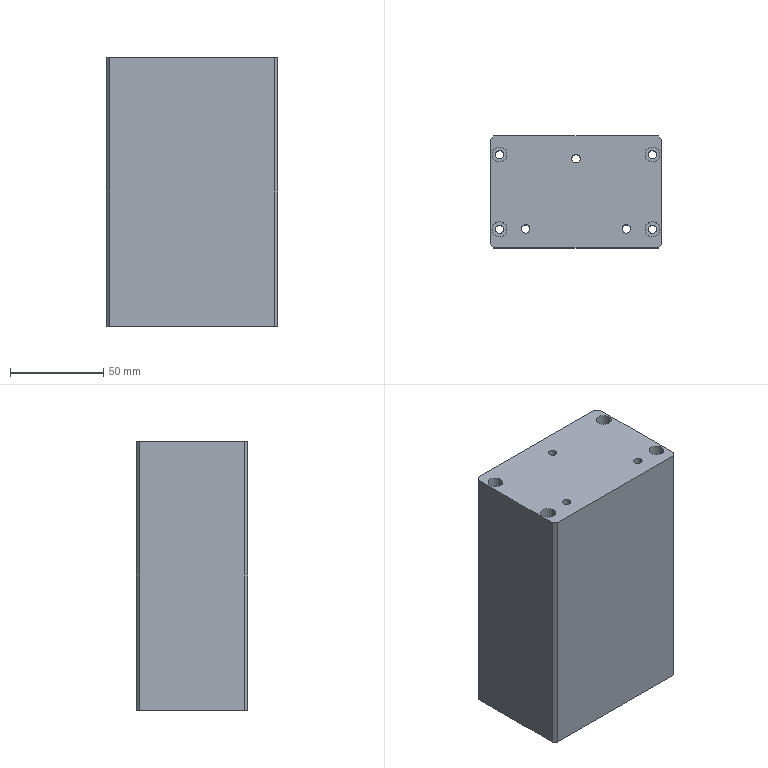Part | SolidWorks | features HoleWzd 2, Chamfer 1, Extrusion 1 | 1 solid | 45 faces | box 92 x 60 x 144 mm | volume 769072 mm3 | cylinder 28 | plane 17 | commonest cylinder face diameters 4.5 x14 8 x14
STEP:
#1=CARTESIAN_POINT('',(4.,17.7,37.));
#2=VERTEX_POINT('',#1);
#3=CARTESIAN_POINT('',(-4.,17.7,37.));
#4=VERTEX_POINT('',#3);
#5=CARTESIAN_POINT('',(0.,17.7,37.));
#6=DIRECTION('',(0.,0.,-1.));
#7=DIRECTION('',(-1.,0.,0.));
#8=AXIS2_PLACEMENT_3D('',#5,#6,#7);
#9=CIRCLE('',#8,4.);
#10=EDGE_CURVE('',#2,#4,#9,.T.);
#11=ORIENTED_EDGE('',*,*,#10,.F.);
#12=CARTESIAN_POINT('',(4.,17.7,0.));
#13=VERTEX_POINT('',#12);
#14=CARTESIAN_POINT('',(4.,17.7,0.));
#15=DIRECTION('',(0.,0.,-1.));
#16=VECTOR('',#15,1000.);
#17=LINE('',#14,#16);
#18=EDGE_CURVE('',#2,#13,#17,.T.);
#19=ORIENTED_EDGE('',*,*,#18,.T.);
#20=CARTESIAN_POINT('',(-4.,17.7,0.));
#21=VERTEX_POINT('',#20);
#22=CARTESIAN_POINT('',(0.,17.7,0.));
#23=DIRECTION('',(0.,0.,-1.));
#24=DIRECTION('',(-1.,0.,0.));
#25=AXIS2_PLACEMENT_3D('',#22,#23,#24);
#26=CIRCLE('',#25,4.);
#27=EDGE_CURVE('',#13,#21,#26,.T.);
#28=ORIENTED_EDGE('',*,*,#27,.T.);
#29=CARTESIAN_POINT('',(-4.,17.7,0.));
#30=DIRECTION('',(0.,0.,-1.));
#31=VECTOR('',#30,1000.);
#32=LINE('',#29,#31);
#33=EDGE_CURVE('',#4,#21,#32,.T.);
#34=ORIENTED_EDGE('',*,*,#33,.F.);
#35=EDGE_LOOP('',(#11,#19,#28,#34));
#36=FACE_OUTER_BOUND('',#35,.T.);
#37=CARTESIAN_POINT('',(0.,17.7,0.));
#38=DIRECTION('',(0.,0.,-1.));
#39=DIRECTION('',(-1.,0.,0.));
#40=AXIS2_PLACEMENT_3D('',#37,#38,#39);
#41=CYLINDRICAL_SURFACE('',#40,4.);
#42=ADVANCED_FACE('',(#36),#41,.F.);
#43=CARTESIAN_POINT('',(2.25,17.7,144.));
#44=VERTEX_POINT('',#43);
#45=CARTESIAN_POINT('',(-2.25,17.7,144.));
#46=VERTEX_POINT('',#45);
#47=CARTESIAN_POINT('',(0.,17.7,144.));
#48=DIRECTION('',(0.,0.,-1.));
#49=DIRECTION('',(-1.,0.,0.));
#50=AXIS2_PLACEMENT_3D('',#47,#48,#49);
#51=CIRCLE('',#50,2.25);
#52=EDGE_CURVE('',#44,#46,#51,.T.);
#53=ORIENTED_EDGE('',*,*,#52,.F.);
#54=CARTESIAN_POINT('',(2.25,17.7,37.));
#55=VERTEX_POINT('',#54);
#56=CARTESIAN_POINT('',(2.25,17.7,0.));
#57=DIRECTION('',(0.,0.,-1.));
#58=VECTOR('',#57,1000.);
#59=LINE('',#56,#58);
#60=EDGE_CURVE('',#44,#55,#59,.T.);
#61=ORIENTED_EDGE('',*,*,#60,.T.);
#62=CARTESIAN_POINT('',(-2.25,17.7,37.));
#63=VERTEX_POINT('',#62);
#64=CARTESIAN_POINT('',(0.,17.7,37.));
#65=DIRECTION('',(0.,0.,-1.));
#66=DIRECTION('',(-1.,0.,0.));
#67=AXIS2_PLACEMENT_3D('',#64,#65,#66);
#68=CIRCLE('',#67,2.25);
#69=EDGE_CURVE('',#55,#63,#68,.T.);
#70=ORIENTED_EDGE('',*,*,#69,.T.);
#71=CARTESIAN_POINT('',(-2.25,17.7,0.));
#72=DIRECTION('',(0.,0.,-1.));
#73=VECTOR('',#72,1000.);
#74=LINE('',#71,#73);
#75=EDGE_CURVE('',#46,#63,#74,.T.);
#76=ORIENTED_EDGE('',*,*,#75,.F.);
#77=EDGE_LOOP('',(#53,#61,#70,#76));
#78=FACE_OUTER_BOUND('',#77,.T.);
#79=CARTESIAN_POINT('',(0.,17.7,0.));
#80=DIRECTION('',(0.,0.,-1.));
#81=DIRECTION('',(-1.,0.,0.));
#82=AXIS2_PLACEMENT_3D('',#79,#80,#81);
#83=CYLINDRICAL_SURFACE('',#82,2.25);
#84=ADVANCED_FACE('',(#78),#83,.F.);
#85=CARTESIAN_POINT('',(31.,-19.9,37.));
#86=VERTEX_POINT('',#85);
#87=CARTESIAN_POINT('',(23.,-19.9,37.));
#88=VERTEX_POINT('',#87);
#89=CARTESIAN_POINT('',(27.,-19.9,37.));
#90=DIRECTION('',(0.,0.,-1.));
#91=DIRECTION('',(-1.,0.,0.));
#92=AXIS2_PLACEMENT_3D('',#89,#90,#91);
#93=CIRCLE('',#92,4.);
#94=EDGE_CURVE('',#86,#88,#93,.T.);
#95=ORIENTED_EDGE('',*,*,#94,.F.);
#96=CARTESIAN_POINT('',(31.,-19.9,0.));
#97=VERTEX_POINT('',#96);
#98=CARTESIAN_POINT('',(31.,-19.9,0.));
#99=DIRECTION('',(0.,0.,-1.));
#100=VECTOR('',#99,1000.);
#101=LINE('',#98,#100);
#102=EDGE_CURVE('',#86,#97,#101,.T.);
#103=ORIENTED_EDGE('',*,*,#102,.T.);
#104=CARTESIAN_POINT('',(23.,-19.9,0.));
#105=VERTEX_POINT('',#104);
#106=CARTESIAN_POINT('',(27.,-19.9,0.));
#107=DIRECTION('',(0.,0.,-1.));
#108=DIRECTION('',(-1.,0.,0.));
#109=AXIS2_PLACEMENT_3D('',#106,#107,#108);
#110=CIRCLE('',#109,4.);
#111=EDGE_CURVE('',#97,#105,#110,.T.);
#112=ORIENTED_EDGE('',*,*,#111,.T.);
#113=CARTESIAN_POINT('',(23.,-19.9,0.));
#114=DIRECTION('',(0.,0.,-1.));
#115=VECTOR('',#114,1000.);
#116=LINE('',#113,#115);
#117=EDGE_CURVE('',#88,#105,#116,.T.);
#118=ORIENTED_EDGE('',*,*,#117,.F.);
#119=EDGE_LOOP('',(#95,#103,#112,#118));
#120=FACE_OUTER_BOUND('',#119,.T.);
#121=CARTESIAN_POINT('',(27.,-19.9,0.));
#122=DIRECTION('',(0.,0.,-1.));
#123=DIRECTION('',(-1.,0.,0.));
#124=AXIS2_PLACEMENT_3D('',#121,#122,#123);
#125=CYLINDRICAL_SURFACE('',#124,4.);
#126=ADVANCED_FACE('',(#120),#125,.F.);
#127=CARTESIAN_POINT('',(29.25,-19.9,144.));
#128=VERTEX_POINT('',#127);
#129=CARTESIAN_POINT('',(24.75,-19.9,144.));
#130=VERTEX_POINT('',#129);
#131=CARTESIAN_POINT('',(27.,-19.9,144.));
#132=DIRECTION('',(0.,0.,-1.));
#133=DIRECTION('',(-1.,0.,0.));
#134=AXIS2_PLACEMENT_3D('',#131,#132,#133);
#135=CIRCLE('',#134,2.25);
#136=EDGE_CURVE('',#128,#130,#135,.T.);
#137=ORIENTED_EDGE('',*,*,#136,.F.);
#138=CARTESIAN_POINT('',(29.25,-19.9,37.));
#139=VERTEX_POINT('',#138);
#140=CARTESIAN_POINT('',(29.25,-19.9,0.));
#141=DIRECTION('',(0.,0.,-1.));
#142=VECTOR('',#141,1000.);
#143=LINE('',#140,#142);
#144=EDGE_CURVE('',#128,#139,#143,.T.);
#145=ORIENTED_EDGE('',*,*,#144,.T.);
#146=CARTESIAN_POINT('',(24.75,-19.9,37.));
#147=VERTEX_POINT('',#146);
#148=CARTESIAN_POINT('',(27.,-19.9,37.));
#149=DIRECTION('',(0.,0.,-1.));
#150=DIRECTION('',(-1.,0.,0.));
#151=AXIS2_PLACEMENT_3D('',#148,#149,#150);
#152=CIRCLE('',#151,2.25);
#153=EDGE_CURVE('',#139,#147,#152,.T.);
#154=ORIENTED_EDGE('',*,*,#153,.T.);
#155=CARTESIAN_POINT('',(24.75,-19.9,0.));
#156=DIRECTION('',(0.,0.,-1.));
#157=VECTOR('',#156,1000.);
#158=LINE('',#155,#157);
#159=EDGE_CURVE('',#130,#147,#158,.T.);
#160=ORIENTED_EDGE('',*,*,#159,.F.);
#161=EDGE_LOOP('',(#137,#145,#154,#160));
#162=FACE_OUTER_BOUND('',#161,.T.);
#163=CARTESIAN_POINT('',(27.,-19.9,0.));
#164=DIRECTION('',(0.,0.,-1.));
#165=DIRECTION('',(-1.,0.,0.));
#166=AXIS2_PLACEMENT_3D('',#163,#164,#165);
#167=CYLINDRICAL_SURFACE('',#166,2.25);
#168=ADVANCED_FACE('',(#162),#167,.F.);
#169=CARTESIAN_POINT('',(-23.,-19.9,37.));
#170=VERTEX_POINT('',#169);
#171=CARTESIAN_POINT('',(-31.,-19.9,37.));
#172=VERTEX_POINT('',#171);
#173=CARTESIAN_POINT('',(-27.,-19.9,37.));
#174=DIRECTION('',(0.,0.,-1.));
#175=DIRECTION('',(-1.,0.,0.));
#176=AXIS2_PLACEMENT_3D('',#173,#174,#175);
#177=CIRCLE('',#176,4.);
#178=EDGE_CURVE('',#170,#172,#177,.T.);
#179=ORIENTED_EDGE('',*,*,#178,.F.);
#180=CARTESIAN_POINT('',(-23.,-19.9,0.));
#181=VERTEX_POINT('',#180);
#182=CARTESIAN_POINT('',(-23.,-19.9,0.));
#183=DIRECTION('',(0.,0.,-1.));
#184=VECTOR('',#183,1000.);
#185=LINE('',#182,#184);
#186=EDGE_CURVE('',#170,#181,#185,.T.);
#187=ORIENTED_EDGE('',*,*,#186,.T.);
#188=CARTESIAN_POINT('',(-31.,-19.9,0.));
#189=VERTEX_POINT('',#188);
#190=CARTESIAN_POINT('',(-27.,-19.9,0.));
#191=DIRECTION('',(0.,0.,-1.));
#192=DIRECTION('',(-1.,0.,0.));
#193=AXIS2_PLACEMENT_3D('',#190,#191,#192);
#194=CIRCLE('',#193,4.);
#195=EDGE_CURVE('',#181,#189,#194,.T.);
#196=ORIENTED_EDGE('',*,*,#195,.T.);
#197=CARTESIAN_POINT('',(-31.,-19.9,0.));
#198=DIRECTION('',(0.,0.,-1.));
#199=VECTOR('',#198,1000.);
#200=LINE('',#197,#199);
#201=EDGE_CURVE('',#172,#189,#200,.T.);
#202=ORIENTED_EDGE('',*,*,#201,.F.);
#203=EDGE_LOOP('',(#179,#187,#196,#202));
#204=FACE_OUTER_BOUND('',#203,.T.);
#205=CARTESIAN_POINT('',(-27.,-19.9,0.));
#206=DIRECTION('',(0.,0.,-1.));
#207=DIRECTION('',(-1.,0.,0.));
#208=AXIS2_PLACEMENT_3D('',#205,#206,#207);
#209=CYLINDRICAL_SURFACE('',#208,4.);
#210=ADVANCED_FACE('',(#204),#209,.F.);
#211=CARTESIAN_POINT('',(-24.75,-19.9,144.));
#212=VERTEX_POINT('',#211);
#213=CARTESIAN_POINT('',(-29.25,-19.9,144.));
#214=VERTEX_POINT('',#213);
#215=CARTESIAN_POINT('',(-27.,-19.9,144.));
#216=DIRECTION('',(0.,0.,-1.));
#217=DIRECTION('',(-1.,0.,0.));
#218=AXIS2_PLACEMENT_3D('',#215,#216,#217);
#219=CIRCLE('',#218,2.25);
#220=EDGE_CURVE('',#212,#214,#219,.T.);
#221=ORIENTED_EDGE('',*,*,#220,.F.);
#222=CARTESIAN_POINT('',(-24.75,-19.9,37.));
#223=VERTEX_POINT('',#222);
#224=CARTESIAN_POINT('',(-24.75,-19.9,0.));
#225=DIRECTION('',(0.,0.,-1.));
#226=VECTOR('',#225,1000.);
#227=LINE('',#224,#226);
#228=EDGE_CURVE('',#212,#223,#227,.T.);
#229=ORIENTED_EDGE('',*,*,#228,.T.);
#230=CARTESIAN_POINT('',(-29.25,-19.9,37.));
#231=VERTEX_POINT('',#230);
#232=CARTESIAN_POINT('',(-27.,-19.9,37.));
#233=DIRECTION('',(0.,0.,-1.));
#234=DIRECTION('',(-1.,0.,0.));
#235=AXIS2_PLACEMENT_3D('',#232,#233,#234);
#236=CIRCLE('',#235,2.25);
#237=EDGE_CURVE('',#223,#231,#236,.T.);
#238=ORIENTED_EDGE('',*,*,#237,.T.);
#239=CARTESIAN_POINT('',(-29.25,-19.9,0.));
#240=DIRECTION('',(0.,0.,-1.));
#241=VECTOR('',#240,1000.);
#242=LINE('',#239,#241);
#243=EDGE_CURVE('',#214,#231,#242,.T.);
#244=ORIENTED_EDGE('',*,*,#243,.F.);
#245=EDGE_LOOP('',(#221,#229,#238,#244));
#246=FACE_OUTER_BOUND('',#245,.T.);
#247=CARTESIAN_POINT('',(-27.,-19.9,0.));
#248=DIRECTION('',(0.,0.,-1.));
#249=DIRECTION('',(-1.,0.,0.));
#250=AXIS2_PLACEMENT_3D('',#247,#248,#249);
#251=CYLINDRICAL_SURFACE('',#250,2.25);
#252=ADVANCED_FACE('',(#246),#251,.F.);
#253=CARTESIAN_POINT('',(-45.,20.,109.));
#254=VERTEX_POINT('',#253);
#255=CARTESIAN_POINT('',(-37.,20.,109.));
#256=VERTEX_POINT('',#255);
#257=CARTESIAN_POINT('',(-41.,20.,109.));
#258=DIRECTION('',(0.,0.,1.));
#259=DIRECTION('',(1.,0.,0.));
#260=AXIS2_PLACEMENT_3D('',#257,#258,#259);
#261=CIRCLE('',#260,4.);
#262=EDGE_CURVE('',#254,#256,#261,.T.);
#263=ORIENTED_EDGE('',*,*,#262,.F.);
#264=CARTESIAN_POINT('',(-45.,20.,144.));
#265=VERTEX_POINT('',#264);
#266=CARTESIAN_POINT('',(-45.,20.,144.));
#267=DIRECTION('',(0.,0.,1.));
#268=VECTOR('',#267,1000.);
#269=LINE('',#266,#268);
#270=EDGE_CURVE('',#254,#265,#269,.T.);
#271=ORIENTED_EDGE('',*,*,#270,.T.);
#272=CARTESIAN_POINT('',(-37.,20.,144.));
#273=VERTEX_POINT('',#272);
#274=CARTESIAN_POINT('',(-41.,20.,144.));
#275=DIRECTION('',(0.,0.,1.));
#276=DIRECTION('',(1.,0.,0.));
#277=AXIS2_PLACEMENT_3D('',#274,#275,#276);
#278=CIRCLE('',#277,4.);
#279=EDGE_CURVE('',#265,#273,#278,.T.);
#280=ORIENTED_EDGE('',*,*,#279,.T.);
#281=CARTESIAN_POINT('',(-37.,20.,144.));
#282=DIRECTION('',(0.,0.,1.));
#283=VECTOR('',#282,1000.);
#284=LINE('',#281,#283);
#285=EDGE_CURVE('',#256,#273,#284,.T.);
#286=ORIENTED_EDGE('',*,*,#285,.F.);
#287=EDGE_LOOP('',(#263,#271,#280,#286));
#288=FACE_OUTER_BOUND('',#287,.T.);
#289=CARTESIAN_POINT('',(-41.,20.,144.));
#290=DIRECTION('',(0.,0.,1.));
#291=DIRECTION('',(1.,0.,0.));
#292=AXIS2_PLACEMENT_3D('',#289,#290,#291);
#293=CYLINDRICAL_SURFACE('',#292,4.);
#294=ADVANCED_FACE('',(#288),#293,.F.);
#295=CARTESIAN_POINT('',(-43.25,20.,0.));
#296=VERTEX_POINT('',#295);
#297=CARTESIAN_POINT('',(-38.75,20.,0.));
#298=VERTEX_POINT('',#297);
#299=CARTESIAN_POINT('',(-41.,20.,0.));
#300=DIRECTION('',(0.,0.,1.));
#301=DIRECTION('',(1.,0.,0.));
#302=AXIS2_PLACEMENT_3D('',#299,#300,#301);
#303=CIRCLE('',#302,2.25);
#304=EDGE_CURVE('',#296,#298,#303,.T.);
#305=ORIENTED_EDGE('',*,*,#304,.F.);
#306=CARTESIAN_POINT('',(-43.25,20.,109.));
#307=VERTEX_POINT('',#306);
#308=CARTESIAN_POINT('',(-43.25,20.,144.));
#309=DIRECTION('',(0.,0.,1.));
#310=VECTOR('',#309,1000.);
#311=LINE('',#308,#310);
#312=EDGE_CURVE('',#296,#307,#311,.T.);
#313=ORIENTED_EDGE('',*,*,#312,.T.);
#314=CARTESIAN_POINT('',(-38.75,20.,109.));
#315=VERTEX_POINT('',#314);
#316=CARTESIAN_POINT('',(-41.,20.,109.));
#317=DIRECTION('',(0.,0.,1.));
#318=DIRECTION('',(1.,0.,0.));
#319=AXIS2_PLACEMENT_3D('',#316,#317,#318);
#320=CIRCLE('',#319,2.25);
#321=EDGE_CURVE('',#307,#315,#320,.T.);
#322=ORIENTED_EDGE('',*,*,#321,.T.);
#323=CARTESIAN_POINT('',(-38.75,20.,144.));
#324=DIRECTION('',(0.,0.,1.));
#325=VECTOR('',#324,1000.);
#326=LINE('',#323,#325);
#327=EDGE_CURVE('',#298,#315,#326,.T.);
#328=ORIENTED_EDGE('',*,*,#327,.F.);
#329=EDGE_LOOP('',(#305,#313,#322,#328));
#330=FACE_OUTER_BOUND('',#329,.T.);
#331=CARTESIAN_POINT('',(-41.,20.,144.));
#332=DIRECTION('',(0.,0.,1.));
#333=DIRECTION('',(1.,0.,0.));
#334=AXIS2_PLACEMENT_3D('',#331,#332,#333);
#335=CYLINDRICAL_SURFACE('',#334,2.25);
#336=ADVANCED_FACE('',(#330),#335,.F.);
#337=CARTESIAN_POINT('',(-45.,-20.,109.));
#338=VERTEX_POINT('',#337);
#339=CARTESIAN_POINT('',(-37.,-20.,109.));
#340=VERTEX_POINT('',#339);
#341=CARTESIAN_POINT('',(-41.,-20.,109.));
#342=DIRECTION('',(0.,0.,1.));
#343=DIRECTION('',(1.,0.,0.));
#344=AXIS2_PLACEMENT_3D('',#341,#342,#343);
#345=CIRCLE('',#344,4.);
#346=EDGE_CURVE('',#338,#340,#345,.T.);
#347=ORIENTED_EDGE('',*,*,#346,.F.);
#348=CARTESIAN_POINT('',(-45.,-20.,144.));
#349=VERTEX_POINT('',#348);
#350=CARTESIAN_POINT('',(-45.,-20.,144.));
#351=DIRECTION('',(0.,0.,1.));
#352=VECTOR('',#351,1000.);
#353=LINE('',#350,#352);
#354=EDGE_CURVE('',#338,#349,#353,.T.);
#355=ORIENTED_EDGE('',*,*,#354,.T.);
#356=CARTESIAN_POINT('',(-37.,-20.,144.));
#357=VERTEX_POINT('',#356);
#358=CARTESIAN_POINT('',(-41.,-20.,144.));
#359=DIRECTION('',(0.,0.,1.));
#360=DIRECTION('',(1.,0.,0.));
#361=AXIS2_PLACEMENT_3D('',#358,#359,#360);
#362=CIRCLE('',#361,4.);
#363=EDGE_CURVE('',#349,#357,#362,.T.);
#364=ORIENTED_EDGE('',*,*,#363,.T.);
#365=CARTESIAN_POINT('',(-37.,-20.,144.));
#366=DIRECTION('',(0.,0.,1.));
#367=VECTOR('',#366,1000.);
#368=LINE('',#365,#367);
#369=EDGE_CURVE('',#340,#357,#368,.T.);
#370=ORIENTED_EDGE('',*,*,#369,.F.);
#371=EDGE_LOOP('',(#347,#355,#364,#370));
#372=FACE_OUTER_BOUND('',#371,.T.);
#373=CARTESIAN_POINT('',(-41.,-20.,144.));
#374=DIRECTION('',(0.,0.,1.));
#375=DIRECTION('',(1.,0.,0.));
#376=AXIS2_PLACEMENT_3D('',#373,#374,#375);
#377=CYLINDRICAL_SURFACE('',#376,4.);
#378=ADVANCED_FACE('',(#372),#377,.F.);
#379=CARTESIAN_POINT('',(-43.25,-20.,0.));
#380=VERTEX_POINT('',#379);
#381=CARTESIAN_POINT('',(-38.75,-20.,0.));
#382=VERTEX_POINT('',#381);
#383=CARTESIAN_POINT('',(-41.,-20.,0.));
#384=DIRECTION('',(0.,0.,1.));
#385=DIRECTION('',(1.,0.,0.));
#386=AXIS2_PLACEMENT_3D('',#383,#384,#385);
#387=CIRCLE('',#386,2.25);
#388=EDGE_CURVE('',#380,#382,#387,.T.);
#389=ORIENTED_EDGE('',*,*,#388,.F.);
#390=CARTESIAN_POINT('',(-43.25,-20.,109.));
#391=VERTEX_POINT('',#390);
#392=CARTESIAN_POINT('',(-43.25,-20.,144.));
#393=DIRECTION('',(0.,0.,1.));
#394=VECTOR('',#393,1000.);
#395=LINE('',#392,#394);
#396=EDGE_CURVE('',#380,#391,#395,.T.);
#397=ORIENTED_EDGE('',*,*,#396,.T.);
#398=CARTESIAN_POINT('',(-38.75,-20.,109.));
#399=VERTEX_POINT('',#398);
#400=CARTESIAN_POINT('',(-41.,-20.,109.));
#401=DIRECTION('',(0.,0.,1.));
#402=DIRECTION('',(1.,0.,0.));
#403=AXIS2_PLACEMENT_3D('',#400,#401,#402);
#404=CIRCLE('',#403,2.25);
#405=EDGE_CURVE('',#391,#399,#404,.T.);
#406=ORIENTED_EDGE('',*,*,#405,.T.);
#407=CARTESIAN_POINT('',(-38.75,-20.,144.));
#408=DIRECTION('',(0.,0.,1.));
#409=VECTOR('',#408,1000.);
#410=LINE('',#407,#409);
#411=EDGE_CURVE('',#382,#399,#410,.T.);
#412=ORIENTED_EDGE('',*,*,#411,.F.);
#413=EDGE_LOOP('',(#389,#397,#406,#412));
#414=FACE_OUTER_BOUND('',#413,.T.);
#415=CARTESIAN_POINT('',(-41.,-20.,144.));
#416=DIRECTION('',(0.,0.,1.));
#417=DIRECTION('',(1.,0.,0.));
#418=AXIS2_PLACEMENT_3D('',#415,#416,#417);
#419=CYLINDRICAL_SURFACE('',#418,2.25);
#420=ADVANCED_FACE('',(#414),#419,.F.);
#421=CARTESIAN_POINT('',(37.,20.,109.));
#422=VERTEX_POINT('',#421);
#423=CARTESIAN_POINT('',(45.,20.,109.));
#424=VERTEX_POINT('',#423);
#425=CARTESIAN_POINT('',(41.,20.,109.));
#426=DIRECTION('',(0.,0.,1.));
#427=DIRECTION('',(1.,0.,0.));
#428=AXIS2_PLACEMENT_3D('',#425,#426,#427);
#429=CIRCLE('',#428,4.);
#430=EDGE_CURVE('',#422,#424,#429,.T.);
#431=ORIENTED_EDGE('',*,*,#430,.F.);
#432=CARTESIAN_POINT('',(37.,20.,144.));
#433=VERTEX_POINT('',#432);
#434=CARTESIAN_POINT('',(37.,20.,144.));
#435=DIRECTION('',(0.,0.,1.));
#436=VECTOR('',#435,1000.);
#437=LINE('',#434,#436);
#438=EDGE_CURVE('',#422,#433,#437,.T.);
#439=ORIENTED_EDGE('',*,*,#438,.T.);
#440=CARTESIAN_POINT('',(45.,20.,144.));
#441=VERTEX_POINT('',#440);
#442=CARTESIAN_POINT('',(41.,20.,144.));
#443=DIRECTION('',(0.,0.,1.));
#444=DIRECTION('',(1.,0.,0.));
#445=AXIS2_PLACEMENT_3D('',#442,#443,#444);
#446=CIRCLE('',#445,4.);
#447=EDGE_CURVE('',#433,#441,#446,.T.);
#448=ORIENTED_EDGE('',*,*,#447,.T.);
#449=CARTESIAN_POINT('',(45.,20.,144.));
#450=DIRECTION('',(0.,0.,1.));
#451=VECTOR('',#450,1000.);
#452=LINE('',#449,#451);
#453=EDGE_CURVE('',#424,#441,#452,.T.);
#454=ORIENTED_EDGE('',*,*,#453,.F.);
#455=EDGE_LOOP('',(#431,#439,#448,#454));
#456=FACE_OUTER_BOUND('',#455,.T.);
#457=CARTESIAN_POINT('',(41.,20.,144.));
#458=DIRECTION('',(0.,0.,1.));
#459=DIRECTION('',(1.,0.,0.));
#460=AXIS2_PLACEMENT_3D('',#457,#458,#459);
#461=CYLINDRICAL_SURFACE('',#460,4.);
#462=ADVANCED_FACE('',(#456),#461,.F.);
#463=CARTESIAN_POINT('',(38.75,20.,0.));
#464=VERTEX_POINT('',#463);
#465=CARTESIAN_POINT('',(43.25,20.,0.));
#466=VERTEX_POINT('',#465);
#467=CARTESIAN_POINT('',(41.,20.,0.));
#468=DIRECTION('',(0.,0.,1.));
#469=DIRECTION('',(1.,0.,0.));
#470=AXIS2_PLACEMENT_3D('',#467,#468,#469);
#471=CIRCLE('',#470,2.25);
#472=EDGE_CURVE('',#464,#466,#471,.T.);
#473=ORIENTED_EDGE('',*,*,#472,.F.);
#474=CARTESIAN_POINT('',(38.75,20.,109.));
#475=VERTEX_POINT('',#474);
#476=CARTESIAN_POINT('',(38.75,20.,144.));
#477=DIRECTION('',(0.,0.,1.));
#478=VECTOR('',#477,1000.);
#479=LINE('',#476,#478);
#480=EDGE_CURVE('',#464,#475,#479,.T.);
#481=ORIENTED_EDGE('',*,*,#480,.T.);
#482=CARTESIAN_POINT('',(43.25,20.,109.));
#483=VERTEX_POINT('',#482);
#484=CARTESIAN_POINT('',(41.,20.,109.));
#485=DIRECTION('',(0.,0.,1.));
#486=DIRECTION('',(1.,0.,0.));
#487=AXIS2_PLACEMENT_3D('',#484,#485,#486);
#488=CIRCLE('',#487,2.25);
#489=EDGE_CURVE('',#475,#483,#488,.T.);
#490=ORIENTED_EDGE('',*,*,#489,.T.);
#491=CARTESIAN_POINT('',(43.25,20.,144.));
#492=DIRECTION('',(0.,0.,1.));
#493=VECTOR('',#492,1000.);
#494=LINE('',#491,#493);
#495=EDGE_CURVE('',#466,#483,#494,.T.);
#496=ORIENTED_EDGE('',*,*,#495,.F.);
#497=EDGE_LOOP('',(#473,#481,#490,#496));
#498=FACE_OUTER_BOUND('',#497,.T.);
#499=CARTESIAN_POINT('',(41.,20.,144.));
#500=DIRECTION('',(0.,0.,1.));
#501=DIRECTION('',(1.,0.,0.));
#502=AXIS2_PLACEMENT_3D('',#499,#500,#501);
#503=CYLINDRICAL_SURFACE('',#502,2.25);
#504=ADVANCED_FACE('',(#498),#503,.F.);
#505=CARTESIAN_POINT('',(37.,-20.,109.));
#506=VERTEX_POINT('',#505);
#507=CARTESIAN_POINT('',(45.,-20.,109.));
#508=VERTEX_POINT('',#507);
#509=CARTESIAN_POINT('',(41.,-20.,109.));
#510=DIRECTION('',(0.,0.,1.));
#511=DIRECTION('',(1.,0.,0.));
#512=AXIS2_PLACEMENT_3D('',#509,#510,#511);
#513=CIRCLE('',#512,4.);
#514=EDGE_CURVE('',#506,#508,#513,.T.);
#515=ORIENTED_EDGE('',*,*,#514,.F.);
#516=CARTESIAN_POINT('',(37.,-20.,144.));
#517=VERTEX_POINT('',#516);
#518=CARTESIAN_POINT('',(37.,-20.,144.));
#519=DIRECTION('',(0.,0.,1.));
#520=VECTOR('',#519,1000.);
#521=LINE('',#518,#520);
#522=EDGE_CURVE('',#506,#517,#521,.T.);
#523=ORIENTED_EDGE('',*,*,#522,.T.);
#524=CARTESIAN_POINT('',(45.,-20.,144.));
#525=VERTEX_POINT('',#524);
#526=CARTESIAN_POINT('',(41.,-20.,144.));
#527=DIRECTION('',(0.,0.,1.));
#528=DIRECTION('',(1.,0.,0.));
#529=AXIS2_PLACEMENT_3D('',#526,#527,#528);
#530=CIRCLE('',#529,4.);
#531=EDGE_CURVE('',#517,#525,#530,.T.);
#532=ORIENTED_EDGE('',*,*,#531,.T.);
#533=CARTESIAN_POINT('',(45.,-20.,144.));
#534=DIRECTION('',(0.,0.,1.));
#535=VECTOR('',#534,1000.);
#536=LINE('',#533,#535);
#537=EDGE_CURVE('',#508,#525,#536,.T.);
#538=ORIENTED_EDGE('',*,*,#537,.F.);
#539=EDGE_LOOP('',(#515,#523,#532,#538));
#540=FACE_OUTER_BOUND('',#539,.T.);
#541=CARTESIAN_POINT('',(41.,-20.,144.));
#542=DIRECTION('',(0.,0.,1.));
#543=DIRECTION('',(1.,0.,0.));
#544=AXIS2_PLACEMENT_3D('',#541,#542,#543);
#545=CYLINDRICAL_SURFACE('',#544,4.);
#546=ADVANCED_FACE('',(#540),#545,.F.);
#547=CARTESIAN_POINT('',(38.75,-20.,0.));
#548=VERTEX_POINT('',#547);
#549=CARTESIAN_POINT('',(43.25,-20.,0.));
#550=VERTEX_POINT('',#549);
#551=CARTESIAN_POINT('',(41.,-20.,0.));
#552=DIRECTION('',(0.,0.,1.));
#553=DIRECTION('',(1.,0.,0.));
#554=AXIS2_PLACEMENT_3D('',#551,#552,#553);
#555=CIRCLE('',#554,2.25);
#556=EDGE_CURVE('',#548,#550,#555,.T.);
#557=ORIENTED_EDGE('',*,*,#556,.F.);
#558=CARTESIAN_POINT('',(38.75,-20.,109.));
#559=VERTEX_POINT('',#558);
#560=CARTESIAN_POINT('',(38.75,-20.,144.));
#561=DIRECTION('',(0.,0.,1.));
#562=VECTOR('',#561,1000.);
#563=LINE('',#560,#562);
#564=EDGE_CURVE('',#548,#559,#563,.T.);
#565=ORIENTED_EDGE('',*,*,#564,.T.);
#566=CARTESIAN_POINT('',(43.25,-20.,109.));
#567=VERTEX_POINT('',#566);
#568=CARTESIAN_POINT('',(41.,-20.,109.));
#569=DIRECTION('',(0.,0.,1.));
#570=DIRECTION('',(1.,0.,0.));
#571=AXIS2_PLACEMENT_3D('',#568,#569,#570);
#572=CIRCLE('',#571,2.25);
#573=EDGE_CURVE('',#559,#567,#572,.T.);
#574=ORIENTED_EDGE('',*,*,#573,.T.);
#575=CARTESIAN_POINT('',(43.25,-20.,144.));
#576=DIRECTION('',(0.,0.,1.));
#577=VECTOR('',#576,1000.);
#578=LINE('',#575,#577);
#579=EDGE_CURVE('',#550,#567,#578,.T.);
#580=ORIENTED_EDGE('',*,*,#579,.F.);
#581=EDGE_LOOP('',(#557,#565,#574,#580));
#582=FACE_OUTER_BOUND('',#581,.T.);
#583=CARTESIAN_POINT('',(41.,-20.,144.));
#584=DIRECTION('',(0.,0.,1.));
#585=DIRECTION('',(1.,0.,0.));
#586=AXIS2_PLACEMENT_3D('',#583,#584,#585);
#587=CYLINDRICAL_SURFACE('',#586,2.25);
#588=ADVANCED_FACE('',(#582),#587,.F.);
#589=CARTESIAN_POINT('',(46.,-28.,144.));
#590=VERTEX_POINT('',#589);
#591=CARTESIAN_POINT('',(46.,28.,144.));
#592=VERTEX_POINT('',#591);
#593=CARTESIAN_POINT('',(46.,30.,144.));
#594=DIRECTION('',(0.,1.,0.));
#595=VECTOR('',#594,1000.);
#596=LINE('',#593,#595);
#597=EDGE_CURVE('',#590,#592,#596,.T.);
#598=ORIENTED_EDGE('',*,*,#597,.F.);
#599=CARTESIAN_POINT('',(46.,-28.,0.));
#600=VERTEX_POINT('',#599);
#601=CARTESIAN_POINT('',(46.,-28.,144.));
#602=DIRECTION('',(0.,0.,-1.));
#603=VECTOR('',#602,1000.);
#604=LINE('',#601,#603);
#605=EDGE_CURVE('',#590,#600,#604,.T.);
#606=ORIENTED_EDGE('',*,*,#605,.T.);
#607=CARTESIAN_POINT('',(46.,28.,0.));
#608=VERTEX_POINT('',#607);
#609=CARTESIAN_POINT('',(46.,30.,0.));
#610=DIRECTION('',(0.,1.,0.));
#611=VECTOR('',#610,1000.);
#612=LINE('',#609,#611);
#613=EDGE_CURVE('',#600,#608,#612,.T.);
#614=ORIENTED_EDGE('',*,*,#613,.T.);
#615=CARTESIAN_POINT('',(46.,28.,144.));
#616=DIRECTION('',(0.,0.,1.));
#617=VECTOR('',#616,1000.);
#618=LINE('',#615,#617);
#619=EDGE_CURVE('',#608,#592,#618,.T.);
#620=ORIENTED_EDGE('',*,*,#619,.T.);
#621=EDGE_LOOP('',(#598,#606,#614,#620));
#622=FACE_OUTER_BOUND('',#621,.T.);
#623=CARTESIAN_POINT('',(46.,30.,144.));
#624=DIRECTION('',(-1.,0.,0.));
#625=DIRECTION('',(0.,0.,1.));
#626=AXIS2_PLACEMENT_3D('',#623,#624,#625);
#627=PLANE('',#626);
#628=ADVANCED_FACE('',(#622),#627,.F.);
#629=CARTESIAN_POINT('',(44.,30.,144.));
#630=VERTEX_POINT('',#629);
#631=CARTESIAN_POINT('',(-44.,30.,144.));
#632=VERTEX_POINT('',#631);
#633=CARTESIAN_POINT('',(-46.,30.,144.));
#634=DIRECTION('',(-1.,0.,0.));
#635=VECTOR('',#634,1000.);
#636=LINE('',#633,#635);
#637=EDGE_CURVE('',#630,#632,#636,.T.);
#638=ORIENTED_EDGE('',*,*,#637,.F.);
#639=CARTESIAN_POINT('',(44.,30.,0.));
#640=VERTEX_POINT('',#639);
#641=CARTESIAN_POINT('',(44.,30.,144.));
#642=DIRECTION('',(0.,0.,-1.));
#643=VECTOR('',#642,1000.);
#644=LINE('',#641,#643);
#645=EDGE_CURVE('',#630,#640,#644,.T.);
#646=ORIENTED_EDGE('',*,*,#645,.T.);
#647=CARTESIAN_POINT('',(-44.,30.,0.));
#648=VERTEX_POINT('',#647);
#649=CARTESIAN_POINT('',(-46.,30.,0.));
#650=DIRECTION('',(-1.,0.,0.));
#651=VECTOR('',#650,1000.);
#652=LINE('',#649,#651);
#653=EDGE_CURVE('',#640,#648,#652,.T.);
#654=ORIENTED_EDGE('',*,*,#653,.T.);
#655=CARTESIAN_POINT('',(-44.,30.,144.));
#656=DIRECTION('',(0.,0.,1.));
#657=VECTOR('',#656,1000.);
#658=LINE('',#655,#657);
#659=EDGE_CURVE('',#648,#632,#658,.T.);
#660=ORIENTED_EDGE('',*,*,#659,.T.);
#661=EDGE_LOOP('',(#638,#646,#654,#660));
#662=FACE_OUTER_BOUND('',#661,.T.);
#663=CARTESIAN_POINT('',(-46.,30.,144.));
#664=DIRECTION('',(0.,-1.,0.));
#665=DIRECTION('',(0.,0.,-1.));
#666=AXIS2_PLACEMENT_3D('',#663,#664,#665);
#667=PLANE('',#666);
#668=ADVANCED_FACE('',(#662),#667,.F.);
#669=CARTESIAN_POINT('',(-46.,28.,0.));
#670=VERTEX_POINT('',#669);
#671=CARTESIAN_POINT('',(-46.,-28.,0.));
#672=VERTEX_POINT('',#671);
#673=CARTESIAN_POINT('',(-46.,30.,0.));
#674=DIRECTION('',(0.,-1.,0.));
#675=VECTOR('',#674,1000.);
#676=LINE('',#673,#675);
#677=EDGE_CURVE('',#670,#672,#676,.T.);
#678=ORIENTED_EDGE('',*,*,#677,.T.);
#679=CARTESIAN_POINT('',(-46.,-28.,144.));
#680=VERTEX_POINT('',#679);
#681=CARTESIAN_POINT('',(-46.,-28.,144.));
#682=DIRECTION('',(0.,0.,1.));
#683=VECTOR('',#682,1000.);
#684=LINE('',#681,#683);
#685=EDGE_CURVE('',#672,#680,#684,.T.);
#686=ORIENTED_EDGE('',*,*,#685,.T.);
#687=CARTESIAN_POINT('',(-46.,28.,144.));
#688=VERTEX_POINT('',#687);
#689=CARTESIAN_POINT('',(-46.,30.,144.));
#690=DIRECTION('',(0.,-1.,0.));
#691=VECTOR('',#690,1000.);
#692=LINE('',#689,#691);
#693=EDGE_CURVE('',#688,#680,#692,.T.);
#694=ORIENTED_EDGE('',*,*,#693,.F.);
#695=CARTESIAN_POINT('',(-46.,28.,144.));
#696=DIRECTION('',(0.,0.,-1.));
#697=VECTOR('',#696,1000.);
#698=LINE('',#695,#697);
#699=EDGE_CURVE('',#688,#670,#698,.T.);
#700=ORIENTED_EDGE('',*,*,#699,.T.);
#701=EDGE_LOOP('',(#678,#686,#694,#700));
#702=FACE_OUTER_BOUND('',#701,.T.);
#703=CARTESIAN_POINT('',(-46.,30.,144.));
#704=DIRECTION('',(1.,0.,0.));
#705=DIRECTION('',(0.,1.,0.));
#706=AXIS2_PLACEMENT_3D('',#703,#704,#705);
#707=PLANE('',#706);
#708=ADVANCED_FACE('',(#702),#707,.F.);
#709=CARTESIAN_POINT('',(-44.,-30.,0.));
#710=VERTEX_POINT('',#709);
#711=CARTESIAN_POINT('',(44.,-30.,0.));
#712=VERTEX_POINT('',#711);
#713=CARTESIAN_POINT('',(-46.,-30.,0.));
#714=DIRECTION('',(1.,0.,0.));
#715=VECTOR('',#714,1000.);
#716=LINE('',#713,#715);
#717=EDGE_CURVE('',#710,#712,#716,.T.);
#718=ORIENTED_EDGE('',*,*,#717,.T.);
#719=CARTESIAN_POINT('',(44.,-30.,144.));
#720=VERTEX_POINT('',#719);
#721=CARTESIAN_POINT('',(44.,-30.,144.));
#722=DIRECTION('',(0.,0.,1.));
#723=VECTOR('',#722,1000.);
#724=LINE('',#721,#723);
#725=EDGE_CURVE('',#712,#720,#724,.T.);
#726=ORIENTED_EDGE('',*,*,#725,.T.);
#727=CARTESIAN_POINT('',(-44.,-30.,144.));
#728=VERTEX_POINT('',#727);
#729=CARTESIAN_POINT('',(-46.,-30.,144.));
#730=DIRECTION('',(1.,0.,0.));
#731=VECTOR('',#730,1000.);
#732=LINE('',#729,#731);
#733=EDGE_CURVE('',#728,#720,#732,.T.);
#734=ORIENTED_EDGE('',*,*,#733,.F.);
#735=CARTESIAN_POINT('',(-44.,-30.,144.));
#736=DIRECTION('',(0.,0.,-1.));
#737=VECTOR('',#736,1000.);
#738=LINE('',#735,#737);
#739=EDGE_CURVE('',#728,#710,#738,.T.);
#740=ORIENTED_EDGE('',*,*,#739,.T.);
#741=EDGE_LOOP('',(#718,#726,#734,#740));
#742=FACE_OUTER_BOUND('',#741,.T.);
#743=CARTESIAN_POINT('',(-46.,-30.,144.));
#744=DIRECTION('',(0.,1.,0.));
#745=DIRECTION('',(0.,0.,1.));
#746=AXIS2_PLACEMENT_3D('',#743,#744,#745);
#747=PLANE('',#746);
#748=ADVANCED_FACE('',(#742),#747,.F.);
#749=CARTESIAN_POINT('',(0.,17.7,144.));
#750=DIRECTION('',(0.,0.,-1.));
#751=DIRECTION('',(-1.,0.,0.));
#752=AXIS2_PLACEMENT_3D('',#749,#750,#751);
#753=CIRCLE('',#752,2.25);
#754=EDGE_CURVE('',#46,#44,#753,.T.);
#755=ORIENTED_EDGE('',*,*,#754,.T.);
#756=ORIENTED_EDGE('',*,*,#52,.T.);
#757=EDGE_LOOP('',(#755,#756));
#758=FACE_BOUND('',#757,.T.);
#759=CARTESIAN_POINT('',(27.,-19.9,144.));
#760=DIRECTION('',(0.,0.,-1.));
#761=DIRECTION('',(-1.,0.,0.));
#762=AXIS2_PLACEMENT_3D('',#759,#760,#761);
#763=CIRCLE('',#762,2.25);
#764=EDGE_CURVE('',#130,#128,#763,.T.);
#765=ORIENTED_EDGE('',*,*,#764,.T.);
#766=ORIENTED_EDGE('',*,*,#136,.T.);
#767=EDGE_LOOP('',(#765,#766));
#768=FACE_BOUND('',#767,.T.);
#769=CARTESIAN_POINT('',(-27.,-19.9,144.));
#770=DIRECTION('',(0.,0.,-1.));
#771=DIRECTION('',(-1.,0.,0.));
#772=AXIS2_PLACEMENT_3D('',#769,#770,#771);
#773=CIRCLE('',#772,2.25);
#774=EDGE_CURVE('',#214,#212,#773,.T.);
#775=ORIENTED_EDGE('',*,*,#774,.T.);
#776=ORIENTED_EDGE('',*,*,#220,.T.);
#777=EDGE_LOOP('',(#775,#776));
#778=FACE_BOUND('',#777,.T.);
#779=CARTESIAN_POINT('',(-41.,20.,144.));
#780=DIRECTION('',(0.,0.,1.));
#781=DIRECTION('',(1.,0.,0.));
#782=AXIS2_PLACEMENT_3D('',#779,#780,#781);
#783=CIRCLE('',#782,4.);
#784=EDGE_CURVE('',#273,#265,#783,.T.);
#785=ORIENTED_EDGE('',*,*,#784,.F.);
#786=ORIENTED_EDGE('',*,*,#279,.F.);
#787=EDGE_LOOP('',(#785,#786));
#788=FACE_BOUND('',#787,.T.);
#789=CARTESIAN_POINT('',(-41.,-20.,144.));
#790=DIRECTION('',(0.,0.,1.));
#791=DIRECTION('',(1.,0.,0.));
#792=AXIS2_PLACEMENT_3D('',#789,#790,#791);
#793=CIRCLE('',#792,4.);
#794=EDGE_CURVE('',#357,#349,#793,.T.);
#795=ORIENTED_EDGE('',*,*,#794,.F.);
#796=ORIENTED_EDGE('',*,*,#363,.F.);
#797=EDGE_LOOP('',(#795,#796));
#798=FACE_BOUND('',#797,.T.);
#799=CARTESIAN_POINT('',(41.,20.,144.));
#800=DIRECTION('',(0.,0.,1.));
#801=DIRECTION('',(1.,0.,0.));
#802=AXIS2_PLACEMENT_3D('',#799,#800,#801);
#803=CIRCLE('',#802,4.);
#804=EDGE_CURVE('',#441,#433,#803,.T.);
#805=ORIENTED_EDGE('',*,*,#804,.F.);
#806=ORIENTED_EDGE('',*,*,#447,.F.);
#807=EDGE_LOOP('',(#805,#806));
#808=FACE_BOUND('',#807,.T.);
#809=CARTESIAN_POINT('',(41.,-20.,144.));
#810=DIRECTION('',(0.,0.,1.));
#811=DIRECTION('',(1.,0.,0.));
#812=AXIS2_PLACEMENT_3D('',#809,#810,#811);
#813=CIRCLE('',#812,4.);
#814=EDGE_CURVE('',#525,#517,#813,.T.);
#815=ORIENTED_EDGE('',*,*,#814,.F.);
#816=ORIENTED_EDGE('',*,*,#531,.F.);
#817=EDGE_LOOP('',(#815,#816));
#818=FACE_BOUND('',#817,.T.);
#819=ORIENTED_EDGE('',*,*,#733,.T.);
#820=CARTESIAN_POINT('',(37.,-37.,144.));
#821=DIRECTION('',(0.7071,0.7071,0.));
#822=VECTOR('',#821,1000.);
#823=LINE('',#820,#822);
#824=EDGE_CURVE('',#720,#590,#823,.T.);
#825=ORIENTED_EDGE('',*,*,#824,.T.);
#826=ORIENTED_EDGE('',*,*,#597,.T.);
#827=CARTESIAN_POINT('',(37.,37.,144.));
#828=DIRECTION('',(-0.7071,0.7071,0.));
#829=VECTOR('',#828,1000.);
#830=LINE('',#827,#829);
#831=EDGE_CURVE('',#592,#630,#830,.T.);
#832=ORIENTED_EDGE('',*,*,#831,.T.);
#833=ORIENTED_EDGE('',*,*,#637,.T.);
#834=CARTESIAN_POINT('',(-37.,37.,144.));
#835=DIRECTION('',(-0.7071,-0.7071,0.));
#836=VECTOR('',#835,1000.);
#837=LINE('',#834,#836);
#838=EDGE_CURVE('',#632,#688,#837,.T.);
#839=ORIENTED_EDGE('',*,*,#838,.T.);
#840=ORIENTED_EDGE('',*,*,#693,.T.);
#841=CARTESIAN_POINT('',(-37.,-37.,144.));
#842=DIRECTION('',(0.7071,-0.7071,0.));
#843=VECTOR('',#842,1000.);
#844=LINE('',#841,#843);
#845=EDGE_CURVE('',#680,#728,#844,.T.);
#846=ORIENTED_EDGE('',*,*,#845,.T.);
#847=EDGE_LOOP('',(#819,#825,#826,#832,#833,#839,#840,#846));
#848=FACE_OUTER_BOUND('',#847,.T.);
#849=CARTESIAN_POINT('',(0.,0.,144.));
#850=DIRECTION('',(0.,0.,1.));
#851=DIRECTION('',(1.,0.,0.));
#852=AXIS2_PLACEMENT_3D('',#849,#850,#851);
#853=PLANE('',#852);
#854=ADVANCED_FACE('',(#758,#768,#778,#788,#798,#808,#818,#848),#853,.T.);
#855=CARTESIAN_POINT('',(0.,17.7,0.));
#856=DIRECTION('',(0.,0.,-1.));
#857=DIRECTION('',(-1.,0.,0.));
#858=AXIS2_PLACEMENT_3D('',#855,#856,#857);
#859=CIRCLE('',#858,4.);
#860=EDGE_CURVE('',#21,#13,#859,.T.);
#861=ORIENTED_EDGE('',*,*,#860,.F.);
#862=ORIENTED_EDGE('',*,*,#27,.F.);
#863=EDGE_LOOP('',(#861,#862));
#864=FACE_BOUND('',#863,.T.);
#865=CARTESIAN_POINT('',(27.,-19.9,0.));
#866=DIRECTION('',(0.,0.,-1.));
#867=DIRECTION('',(-1.,0.,0.));
#868=AXIS2_PLACEMENT_3D('',#865,#866,#867);
#869=CIRCLE('',#868,4.);
#870=EDGE_CURVE('',#105,#97,#869,.T.);
#871=ORIENTED_EDGE('',*,*,#870,.F.);
#872=ORIENTED_EDGE('',*,*,#111,.F.);
#873=EDGE_LOOP('',(#871,#872));
#874=FACE_BOUND('',#873,.T.);
#875=CARTESIAN_POINT('',(-27.,-19.9,0.));
#876=DIRECTION('',(0.,0.,-1.));
#877=DIRECTION('',(-1.,0.,0.));
#878=AXIS2_PLACEMENT_3D('',#875,#876,#877);
#879=CIRCLE('',#878,4.);
#880=EDGE_CURVE('',#189,#181,#879,.T.);
#881=ORIENTED_EDGE('',*,*,#880,.F.);
#882=ORIENTED_EDGE('',*,*,#195,.F.);
#883=EDGE_LOOP('',(#881,#882));
#884=FACE_BOUND('',#883,.T.);
#885=CARTESIAN_POINT('',(-41.,20.,0.));
#886=DIRECTION('',(0.,0.,1.));
#887=DIRECTION('',(1.,0.,0.));
#888=AXIS2_PLACEMENT_3D('',#885,#886,#887);
#889=CIRCLE('',#888,2.25);
#890=EDGE_CURVE('',#298,#296,#889,.T.);
#891=ORIENTED_EDGE('',*,*,#890,.T.);
#892=ORIENTED_EDGE('',*,*,#304,.T.);
#893=EDGE_LOOP('',(#891,#892));
#894=FACE_BOUND('',#893,.T.);
#895=CARTESIAN_POINT('',(-41.,-20.,0.));
#896=DIRECTION('',(0.,0.,1.));
#897=DIRECTION('',(1.,0.,0.));
#898=AXIS2_PLACEMENT_3D('',#895,#896,#897);
#899=CIRCLE('',#898,2.25);
#900=EDGE_CURVE('',#382,#380,#899,.T.);
#901=ORIENTED_EDGE('',*,*,#900,.T.);
#902=ORIENTED_EDGE('',*,*,#388,.T.);
#903=EDGE_LOOP('',(#901,#902));
#904=FACE_BOUND('',#903,.T.);
#905=CARTESIAN_POINT('',(41.,20.,0.));
#906=DIRECTION('',(0.,0.,1.));
#907=DIRECTION('',(1.,0.,0.));
#908=AXIS2_PLACEMENT_3D('',#905,#906,#907);
#909=CIRCLE('',#908,2.25);
#910=EDGE_CURVE('',#466,#464,#909,.T.);
#911=ORIENTED_EDGE('',*,*,#910,.T.);
#912=ORIENTED_EDGE('',*,*,#472,.T.);
#913=EDGE_LOOP('',(#911,#912));
#914=FACE_BOUND('',#913,.T.);
#915=CARTESIAN_POINT('',(41.,-20.,0.));
#916=DIRECTION('',(0.,0.,1.));
#917=DIRECTION('',(1.,0.,0.));
#918=AXIS2_PLACEMENT_3D('',#915,#916,#917);
#919=CIRCLE('',#918,2.25);
#920=EDGE_CURVE('',#550,#548,#919,.T.);
#921=ORIENTED_EDGE('',*,*,#920,.T.);
#922=ORIENTED_EDGE('',*,*,#556,.T.);
#923=EDGE_LOOP('',(#921,#922));
#924=FACE_BOUND('',#923,.T.);
#925=ORIENTED_EDGE('',*,*,#613,.F.);
#926=CARTESIAN_POINT('',(46.,-28.,0.));
#927=DIRECTION('',(-0.7071,-0.7071,0.));
#928=VECTOR('',#927,1000.);
#929=LINE('',#926,#928);
#930=EDGE_CURVE('',#600,#712,#929,.T.);
#931=ORIENTED_EDGE('',*,*,#930,.T.);
#932=ORIENTED_EDGE('',*,*,#717,.F.);
#933=CARTESIAN_POINT('',(-44.,-30.,0.));
#934=DIRECTION('',(-0.7071,0.7071,0.));
#935=VECTOR('',#934,1000.);
#936=LINE('',#933,#935);
#937=EDGE_CURVE('',#710,#672,#936,.T.);
#938=ORIENTED_EDGE('',*,*,#937,.T.);
#939=ORIENTED_EDGE('',*,*,#677,.F.);
#940=CARTESIAN_POINT('',(-46.,28.,0.));
#941=DIRECTION('',(0.7071,0.7071,0.));
#942=VECTOR('',#941,1000.);
#943=LINE('',#940,#942);
#944=EDGE_CURVE('',#670,#648,#943,.T.);
#945=ORIENTED_EDGE('',*,*,#944,.T.);
#946=ORIENTED_EDGE('',*,*,#653,.F.);
#947=CARTESIAN_POINT('',(44.,30.,0.));
#948=DIRECTION('',(0.7071,-0.7071,0.));
#949=VECTOR('',#948,1000.);
#950=LINE('',#947,#949);
#951=EDGE_CURVE('',#640,#608,#950,.T.);
#952=ORIENTED_EDGE('',*,*,#951,.T.);
#953=EDGE_LOOP('',(#925,#931,#932,#938,#939,#945,#946,#952));
#954=FACE_OUTER_BOUND('',#953,.T.);
#955=CARTESIAN_POINT('',(0.,0.,0.));
#956=DIRECTION('',(0.,0.,1.));
#957=DIRECTION('',(1.,0.,0.));
#958=AXIS2_PLACEMENT_3D('',#955,#956,#957);
#959=PLANE('',#958);
#960=ADVANCED_FACE('',(#864,#874,#884,#894,#904,#914,#924,#954),#959,.F.);
#961=ORIENTED_EDGE('',*,*,#564,.F.);
#962=ORIENTED_EDGE('',*,*,#920,.F.);
#963=ORIENTED_EDGE('',*,*,#579,.T.);
#964=CARTESIAN_POINT('',(41.,-20.,109.));
#965=DIRECTION('',(0.,0.,1.));
#966=DIRECTION('',(1.,0.,0.));
#967=AXIS2_PLACEMENT_3D('',#964,#965,#966);
#968=CIRCLE('',#967,2.25);
#969=EDGE_CURVE('',#567,#559,#968,.T.);
#970=ORIENTED_EDGE('',*,*,#969,.T.);
#971=EDGE_LOOP('',(#961,#962,#963,#970));
#972=FACE_OUTER_BOUND('',#971,.T.);
#973=CARTESIAN_POINT('',(41.,-20.,144.));
#974=DIRECTION('',(0.,0.,1.));
#975=DIRECTION('',(1.,0.,0.));
#976=AXIS2_PLACEMENT_3D('',#973,#974,#975);
#977=CYLINDRICAL_SURFACE('',#976,2.25);
#978=ADVANCED_FACE('',(#972),#977,.F.);
#979=ORIENTED_EDGE('',*,*,#969,.F.);
#980=ORIENTED_EDGE('',*,*,#573,.F.);
#981=EDGE_LOOP('',(#979,#980));
#982=FACE_BOUND('',#981,.T.);
#983=CARTESIAN_POINT('',(41.,-20.,109.));
#984=DIRECTION('',(0.,0.,1.));
#985=DIRECTION('',(1.,0.,0.));
#986=AXIS2_PLACEMENT_3D('',#983,#984,#985);
#987=CIRCLE('',#986,4.);
#988=EDGE_CURVE('',#508,#506,#987,.T.);
#989=ORIENTED_EDGE('',*,*,#988,.T.);
#990=ORIENTED_EDGE('',*,*,#514,.T.);
#991=EDGE_LOOP('',(#989,#990));
#992=FACE_OUTER_BOUND('',#991,.T.);
#993=CARTESIAN_POINT('',(43.25,-20.,109.));
#994=DIRECTION('',(0.,0.,-1.));
#995=DIRECTION('',(-1.,0.,0.));
#996=AXIS2_PLACEMENT_3D('',#993,#994,#995);
#997=PLANE('',#996);
#998=ADVANCED_FACE('',(#982,#992),#997,.F.);
#999=ORIENTED_EDGE('',*,*,#522,.F.);
#1000=ORIENTED_EDGE('',*,*,#988,.F.);
#1001=ORIENTED_EDGE('',*,*,#537,.T.);
#1002=ORIENTED_EDGE('',*,*,#814,.T.);
#1003=EDGE_LOOP('',(#999,#1000,#1001,#1002));
#1004=FACE_OUTER_BOUND('',#1003,.T.);
#1005=CARTESIAN_POINT('',(41.,-20.,144.));
#1006=DIRECTION('',(0.,0.,1.));
#1007=DIRECTION('',(1.,0.,0.));
#1008=AXIS2_PLACEMENT_3D('',#1005,#1006,#1007);
#1009=CYLINDRICAL_SURFACE('',#1008,4.);
#1010=ADVANCED_FACE('',(#1004),#1009,.F.);
#1011=ORIENTED_EDGE('',*,*,#480,.F.);
#1012=ORIENTED_EDGE('',*,*,#910,.F.);
#1013=ORIENTED_EDGE('',*,*,#495,.T.);
#1014=CARTESIAN_POINT('',(41.,20.,109.));
#1015=DIRECTION('',(0.,0.,1.));
#1016=DIRECTION('',(1.,0.,0.));
#1017=AXIS2_PLACEMENT_3D('',#1014,#1015,#1016);
#1018=CIRCLE('',#1017,2.25);
#1019=EDGE_CURVE('',#483,#475,#1018,.T.);
#1020=ORIENTED_EDGE('',*,*,#1019,.T.);
#1021=EDGE_LOOP('',(#1011,#1012,#1013,#1020));
#1022=FACE_OUTER_BOUND('',#1021,.T.);
#1023=CARTESIAN_POINT('',(41.,20.,144.));
#1024=DIRECTION('',(0.,0.,1.));
#1025=DIRECTION('',(1.,0.,0.));
#1026=AXIS2_PLACEMENT_3D('',#1023,#1024,#1025);
#1027=CYLINDRICAL_SURFACE('',#1026,2.25);
#1028=ADVANCED_FACE('',(#1022),#1027,.F.);
#1029=ORIENTED_EDGE('',*,*,#1019,.F.);
#1030=ORIENTED_EDGE('',*,*,#489,.F.);
#1031=EDGE_LOOP('',(#1029,#1030));
#1032=FACE_BOUND('',#1031,.T.);
#1033=CARTESIAN_POINT('',(41.,20.,109.));
#1034=DIRECTION('',(0.,0.,1.));
#1035=DIRECTION('',(1.,0.,0.));
#1036=AXIS2_PLACEMENT_3D('',#1033,#1034,#1035);
#1037=CIRCLE('',#1036,4.);
#1038=EDGE_CURVE('',#424,#422,#1037,.T.);
#1039=ORIENTED_EDGE('',*,*,#1038,.T.);
#1040=ORIENTED_EDGE('',*,*,#430,.T.);
#1041=EDGE_LOOP('',(#1039,#1040));
#1042=FACE_OUTER_BOUND('',#1041,.T.);
#1043=CARTESIAN_POINT('',(43.25,20.,109.));
#1044=DIRECTION('',(0.,0.,-1.));
#1045=DIRECTION('',(-1.,0.,0.));
#1046=AXIS2_PLACEMENT_3D('',#1043,#1044,#1045);
#1047=PLANE('',#1046);
#1048=ADVANCED_FACE('',(#1032,#1042),#1047,.F.);
#1049=ORIENTED_EDGE('',*,*,#438,.F.);
#1050=ORIENTED_EDGE('',*,*,#1038,.F.);
#1051=ORIENTED_EDGE('',*,*,#453,.T.);
#1052=ORIENTED_EDGE('',*,*,#804,.T.);
#1053=EDGE_LOOP('',(#1049,#1050,#1051,#1052));
#1054=FACE_OUTER_BOUND('',#1053,.T.);
#1055=CARTESIAN_POINT('',(41.,20.,144.));
#1056=DIRECTION('',(0.,0.,1.));
#1057=DIRECTION('',(1.,0.,0.));
#1058=AXIS2_PLACEMENT_3D('',#1055,#1056,#1057);
#1059=CYLINDRICAL_SURFACE('',#1058,4.);
#1060=ADVANCED_FACE('',(#1054),#1059,.F.);
#1061=ORIENTED_EDGE('',*,*,#396,.F.);
#1062=ORIENTED_EDGE('',*,*,#900,.F.);
#1063=ORIENTED_EDGE('',*,*,#411,.T.);
#1064=CARTESIAN_POINT('',(-41.,-20.,109.));
#1065=DIRECTION('',(0.,0.,1.));
#1066=DIRECTION('',(1.,0.,0.));
#1067=AXIS2_PLACEMENT_3D('',#1064,#1065,#1066);
#1068=CIRCLE('',#1067,2.25);
#1069=EDGE_CURVE('',#399,#391,#1068,.T.);
#1070=ORIENTED_EDGE('',*,*,#1069,.T.);
#1071=EDGE_LOOP('',(#1061,#1062,#1063,#1070));
#1072=FACE_OUTER_BOUND('',#1071,.T.);
#1073=CARTESIAN_POINT('',(-41.,-20.,144.));
#1074=DIRECTION('',(0.,0.,1.));
#1075=DIRECTION('',(1.,0.,0.));
#1076=AXIS2_PLACEMENT_3D('',#1073,#1074,#1075);
#1077=CYLINDRICAL_SURFACE('',#1076,2.25);
#1078=ADVANCED_FACE('',(#1072),#1077,.F.);
#1079=ORIENTED_EDGE('',*,*,#1069,.F.);
#1080=ORIENTED_EDGE('',*,*,#405,.F.);
#1081=EDGE_LOOP('',(#1079,#1080));
#1082=FACE_BOUND('',#1081,.T.);
#1083=CARTESIAN_POINT('',(-41.,-20.,109.));
#1084=DIRECTION('',(0.,0.,1.));
#1085=DIRECTION('',(1.,0.,0.));
#1086=AXIS2_PLACEMENT_3D('',#1083,#1084,#1085);
#1087=CIRCLE('',#1086,4.);
#1088=EDGE_CURVE('',#340,#338,#1087,.T.);
#1089=ORIENTED_EDGE('',*,*,#1088,.T.);
#1090=ORIENTED_EDGE('',*,*,#346,.T.);
#1091=EDGE_LOOP('',(#1089,#1090));
#1092=FACE_OUTER_BOUND('',#1091,.T.);
#1093=CARTESIAN_POINT('',(-38.75,-20.,109.));
#1094=DIRECTION('',(0.,0.,-1.));
#1095=DIRECTION('',(-1.,0.,0.));
#1096=AXIS2_PLACEMENT_3D('',#1093,#1094,#1095);
#1097=PLANE('',#1096);
#1098=ADVANCED_FACE('',(#1082,#1092),#1097,.F.);
#1099=ORIENTED_EDGE('',*,*,#354,.F.);
#1100=ORIENTED_EDGE('',*,*,#1088,.F.);
#1101=ORIENTED_EDGE('',*,*,#369,.T.);
#1102=ORIENTED_EDGE('',*,*,#794,.T.);
#1103=EDGE_LOOP('',(#1099,#1100,#1101,#1102));
#1104=FACE_OUTER_BOUND('',#1103,.T.);
#1105=CARTESIAN_POINT('',(-41.,-20.,144.));
#1106=DIRECTION('',(0.,0.,1.));
#1107=DIRECTION('',(1.,0.,0.));
#1108=AXIS2_PLACEMENT_3D('',#1105,#1106,#1107);
#1109=CYLINDRICAL_SURFACE('',#1108,4.);
#1110=ADVANCED_FACE('',(#1104),#1109,.F.);
#1111=ORIENTED_EDGE('',*,*,#312,.F.);
#1112=ORIENTED_EDGE('',*,*,#890,.F.);
#1113=ORIENTED_EDGE('',*,*,#327,.T.);
#1114=CARTESIAN_POINT('',(-41.,20.,109.));
#1115=DIRECTION('',(0.,0.,1.));
#1116=DIRECTION('',(1.,0.,0.));
#1117=AXIS2_PLACEMENT_3D('',#1114,#1115,#1116);
#1118=CIRCLE('',#1117,2.25);
#1119=EDGE_CURVE('',#315,#307,#1118,.T.);
#1120=ORIENTED_EDGE('',*,*,#1119,.T.);
#1121=EDGE_LOOP('',(#1111,#1112,#1113,#1120));
#1122=FACE_OUTER_BOUND('',#1121,.T.);
#1123=CARTESIAN_POINT('',(-41.,20.,144.));
#1124=DIRECTION('',(0.,0.,1.));
#1125=DIRECTION('',(1.,0.,0.));
#1126=AXIS2_PLACEMENT_3D('',#1123,#1124,#1125);
#1127=CYLINDRICAL_SURFACE('',#1126,2.25);
#1128=ADVANCED_FACE('',(#1122),#1127,.F.);
#1129=ORIENTED_EDGE('',*,*,#1119,.F.);
#1130=ORIENTED_EDGE('',*,*,#321,.F.);
#1131=EDGE_LOOP('',(#1129,#1130));
#1132=FACE_BOUND('',#1131,.T.);
#1133=CARTESIAN_POINT('',(-41.,20.,109.));
#1134=DIRECTION('',(0.,0.,1.));
#1135=DIRECTION('',(1.,0.,0.));
#1136=AXIS2_PLACEMENT_3D('',#1133,#1134,#1135);
#1137=CIRCLE('',#1136,4.);
#1138=EDGE_CURVE('',#256,#254,#1137,.T.);
#1139=ORIENTED_EDGE('',*,*,#1138,.T.);
#1140=ORIENTED_EDGE('',*,*,#262,.T.);
#1141=EDGE_LOOP('',(#1139,#1140));
#1142=FACE_OUTER_BOUND('',#1141,.T.);
#1143=CARTESIAN_POINT('',(-38.75,20.,109.));
#1144=DIRECTION('',(0.,0.,-1.));
#1145=DIRECTION('',(-1.,0.,0.));
#1146=AXIS2_PLACEMENT_3D('',#1143,#1144,#1145);
#1147=PLANE('',#1146);
#1148=ADVANCED_FACE('',(#1132,#1142),#1147,.F.);
#1149=ORIENTED_EDGE('',*,*,#270,.F.);
#1150=ORIENTED_EDGE('',*,*,#1138,.F.);
#1151=ORIENTED_EDGE('',*,*,#285,.T.);
#1152=ORIENTED_EDGE('',*,*,#784,.T.);
#1153=EDGE_LOOP('',(#1149,#1150,#1151,#1152));
#1154=FACE_OUTER_BOUND('',#1153,.T.);
#1155=CARTESIAN_POINT('',(-41.,20.,144.));
#1156=DIRECTION('',(0.,0.,1.));
#1157=DIRECTION('',(1.,0.,0.));
#1158=AXIS2_PLACEMENT_3D('',#1155,#1156,#1157);
#1159=CYLINDRICAL_SURFACE('',#1158,4.);
#1160=ADVANCED_FACE('',(#1154),#1159,.F.);
#1161=ORIENTED_EDGE('',*,*,#824,.F.);
#1162=ORIENTED_EDGE('',*,*,#725,.F.);
#1163=ORIENTED_EDGE('',*,*,#930,.F.);
#1164=ORIENTED_EDGE('',*,*,#605,.F.);
#1165=EDGE_LOOP('',(#1161,#1162,#1163,#1164));
#1166=FACE_OUTER_BOUND('',#1165,.T.);
#1167=CARTESIAN_POINT('',(46.,-28.,144.));
#1168=DIRECTION('',(-0.7071,0.7071,0.));
#1169=DIRECTION('',(0.,0.,-1.));
#1170=AXIS2_PLACEMENT_3D('',#1167,#1168,#1169);
#1171=PLANE('',#1170);
#1172=ADVANCED_FACE('',(#1166),#1171,.F.);
#1173=ORIENTED_EDGE('',*,*,#831,.F.);
#1174=ORIENTED_EDGE('',*,*,#619,.F.);
#1175=ORIENTED_EDGE('',*,*,#951,.F.);
#1176=ORIENTED_EDGE('',*,*,#645,.F.);
#1177=EDGE_LOOP('',(#1173,#1174,#1175,#1176));
#1178=FACE_OUTER_BOUND('',#1177,.T.);
#1179=CARTESIAN_POINT('',(44.,30.,144.));
#1180=DIRECTION('',(-0.7071,-0.7071,0.));
#1181=DIRECTION('',(0.,0.,-1.));
#1182=AXIS2_PLACEMENT_3D('',#1179,#1180,#1181);
#1183=PLANE('',#1182);
#1184=ADVANCED_FACE('',(#1178),#1183,.F.);
#1185=ORIENTED_EDGE('',*,*,#845,.F.);
#1186=ORIENTED_EDGE('',*,*,#685,.F.);
#1187=ORIENTED_EDGE('',*,*,#937,.F.);
#1188=ORIENTED_EDGE('',*,*,#739,.F.);
#1189=EDGE_LOOP('',(#1185,#1186,#1187,#1188));
#1190=FACE_OUTER_BOUND('',#1189,.T.);
#1191=CARTESIAN_POINT('',(-44.,-30.,144.));
#1192=DIRECTION('',(0.7071,0.7071,0.));
#1193=DIRECTION('',(0.,0.,-1.));
#1194=AXIS2_PLACEMENT_3D('',#1191,#1192,#1193);
#1195=PLANE('',#1194);
#1196=ADVANCED_FACE('',(#1190),#1195,.F.);
#1197=ORIENTED_EDGE('',*,*,#838,.F.);
#1198=ORIENTED_EDGE('',*,*,#659,.F.);
#1199=ORIENTED_EDGE('',*,*,#944,.F.);
#1200=ORIENTED_EDGE('',*,*,#699,.F.);
#1201=EDGE_LOOP('',(#1197,#1198,#1199,#1200));
#1202=FACE_OUTER_BOUND('',#1201,.T.);
#1203=CARTESIAN_POINT('',(-46.,28.,144.));
#1204=DIRECTION('',(0.7071,-0.7071,0.));
#1205=DIRECTION('',(0.,0.,-1.));
#1206=AXIS2_PLACEMENT_3D('',#1203,#1204,#1205);
#1207=PLANE('',#1206);
#1208=ADVANCED_FACE('',(#1202),#1207,.F.);
#1209=ORIENTED_EDGE('',*,*,#228,.F.);
#1210=ORIENTED_EDGE('',*,*,#774,.F.);
#1211=ORIENTED_EDGE('',*,*,#243,.T.);
#1212=CARTESIAN_POINT('',(-27.,-19.9,37.));
#1213=DIRECTION('',(0.,0.,-1.));
#1214=DIRECTION('',(-1.,0.,0.));
#1215=AXIS2_PLACEMENT_3D('',#1212,#1213,#1214);
#1216=CIRCLE('',#1215,2.25);
#1217=EDGE_CURVE('',#231,#223,#1216,.T.);
#1218=ORIENTED_EDGE('',*,*,#1217,.T.);
#1219=EDGE_LOOP('',(#1209,#1210,#1211,#1218));
#1220=FACE_OUTER_BOUND('',#1219,.T.);
#1221=CARTESIAN_POINT('',(-27.,-19.9,0.));
#1222=DIRECTION('',(0.,0.,-1.));
#1223=DIRECTION('',(-1.,0.,0.));
#1224=AXIS2_PLACEMENT_3D('',#1221,#1222,#1223);
#1225=CYLINDRICAL_SURFACE('',#1224,2.25);
#1226=ADVANCED_FACE('',(#1220),#1225,.F.);
#1227=ORIENTED_EDGE('',*,*,#1217,.F.);
#1228=ORIENTED_EDGE('',*,*,#237,.F.);
#1229=EDGE_LOOP('',(#1227,#1228));
#1230=FACE_BOUND('',#1229,.T.);
#1231=CARTESIAN_POINT('',(-27.,-19.9,37.));
#1232=DIRECTION('',(0.,0.,-1.));
#1233=DIRECTION('',(-1.,0.,0.));
#1234=AXIS2_PLACEMENT_3D('',#1231,#1232,#1233);
#1235=CIRCLE('',#1234,4.);
#1236=EDGE_CURVE('',#172,#170,#1235,.T.);
#1237=ORIENTED_EDGE('',*,*,#1236,.T.);
#1238=ORIENTED_EDGE('',*,*,#178,.T.);
#1239=EDGE_LOOP('',(#1237,#1238));
#1240=FACE_OUTER_BOUND('',#1239,.T.);
#1241=CARTESIAN_POINT('',(-24.75,-19.9,37.));
#1242=DIRECTION('',(0.,0.,1.));
#1243=DIRECTION('',(1.,0.,0.));
#1244=AXIS2_PLACEMENT_3D('',#1241,#1242,#1243);
#1245=PLANE('',#1244);
#1246=ADVANCED_FACE('',(#1230,#1240),#1245,.F.);
#1247=ORIENTED_EDGE('',*,*,#186,.F.);
#1248=ORIENTED_EDGE('',*,*,#1236,.F.);
#1249=ORIENTED_EDGE('',*,*,#201,.T.);
#1250=ORIENTED_EDGE('',*,*,#880,.T.);
#1251=EDGE_LOOP('',(#1247,#1248,#1249,#1250));
#1252=FACE_OUTER_BOUND('',#1251,.T.);
#1253=CARTESIAN_POINT('',(-27.,-19.9,0.));
#1254=DIRECTION('',(0.,0.,-1.));
#1255=DIRECTION('',(-1.,0.,0.));
#1256=AXIS2_PLACEMENT_3D('',#1253,#1254,#1255);
#1257=CYLINDRICAL_SURFACE('',#1256,4.);
#1258=ADVANCED_FACE('',(#1252),#1257,.F.);
#1259=ORIENTED_EDGE('',*,*,#144,.F.);
#1260=ORIENTED_EDGE('',*,*,#764,.F.);
#1261=ORIENTED_EDGE('',*,*,#159,.T.);
#1262=CARTESIAN_POINT('',(27.,-19.9,37.));
#1263=DIRECTION('',(0.,0.,-1.));
#1264=DIRECTION('',(-1.,0.,0.));
#1265=AXIS2_PLACEMENT_3D('',#1262,#1263,#1264);
#1266=CIRCLE('',#1265,2.25);
#1267=EDGE_CURVE('',#147,#139,#1266,.T.);
#1268=ORIENTED_EDGE('',*,*,#1267,.T.);
#1269=EDGE_LOOP('',(#1259,#1260,#1261,#1268));
#1270=FACE_OUTER_BOUND('',#1269,.T.);
#1271=CARTESIAN_POINT('',(27.,-19.9,0.));
#1272=DIRECTION('',(0.,0.,-1.));
#1273=DIRECTION('',(-1.,0.,0.));
#1274=AXIS2_PLACEMENT_3D('',#1271,#1272,#1273);
#1275=CYLINDRICAL_SURFACE('',#1274,2.25);
#1276=ADVANCED_FACE('',(#1270),#1275,.F.);
#1277=ORIENTED_EDGE('',*,*,#1267,.F.);
#1278=ORIENTED_EDGE('',*,*,#153,.F.);
#1279=EDGE_LOOP('',(#1277,#1278));
#1280=FACE_BOUND('',#1279,.T.);
#1281=CARTESIAN_POINT('',(27.,-19.9,37.));
#1282=DIRECTION('',(0.,0.,-1.));
#1283=DIRECTION('',(-1.,0.,0.));
#1284=AXIS2_PLACEMENT_3D('',#1281,#1282,#1283);
#1285=CIRCLE('',#1284,4.);
#1286=EDGE_CURVE('',#88,#86,#1285,.T.);
#1287=ORIENTED_EDGE('',*,*,#1286,.T.);
#1288=ORIENTED_EDGE('',*,*,#94,.T.);
#1289=EDGE_LOOP('',(#1287,#1288));
#1290=FACE_OUTER_BOUND('',#1289,.T.);
#1291=CARTESIAN_POINT('',(29.25,-19.9,37.));
#1292=DIRECTION('',(0.,0.,1.));
#1293=DIRECTION('',(1.,0.,0.));
#1294=AXIS2_PLACEMENT_3D('',#1291,#1292,#1293);
#1295=PLANE('',#1294);
#1296=ADVANCED_FACE('',(#1280,#1290),#1295,.F.);
#1297=ORIENTED_EDGE('',*,*,#102,.F.);
#1298=ORIENTED_EDGE('',*,*,#1286,.F.);
#1299=ORIENTED_EDGE('',*,*,#117,.T.);
#1300=ORIENTED_EDGE('',*,*,#870,.T.);
#1301=EDGE_LOOP('',(#1297,#1298,#1299,#1300));
#1302=FACE_OUTER_BOUND('',#1301,.T.);
#1303=CARTESIAN_POINT('',(27.,-19.9,0.));
#1304=DIRECTION('',(0.,0.,-1.));
#1305=DIRECTION('',(-1.,0.,0.));
#1306=AXIS2_PLACEMENT_3D('',#1303,#1304,#1305);
#1307=CYLINDRICAL_SURFACE('',#1306,4.);
#1308=ADVANCED_FACE('',(#1302),#1307,.F.);
#1309=ORIENTED_EDGE('',*,*,#60,.F.);
#1310=ORIENTED_EDGE('',*,*,#754,.F.);
#1311=ORIENTED_EDGE('',*,*,#75,.T.);
#1312=CARTESIAN_POINT('',(0.,17.7,37.));
#1313=DIRECTION('',(0.,0.,-1.));
#1314=DIRECTION('',(-1.,0.,0.));
#1315=AXIS2_PLACEMENT_3D('',#1312,#1313,#1314);
#1316=CIRCLE('',#1315,2.25);
#1317=EDGE_CURVE('',#63,#55,#1316,.T.);
#1318=ORIENTED_EDGE('',*,*,#1317,.T.);
#1319=EDGE_LOOP('',(#1309,#1310,#1311,#1318));
#1320=FACE_OUTER_BOUND('',#1319,.T.);
#1321=CARTESIAN_POINT('',(0.,17.7,0.));
#1322=DIRECTION('',(0.,0.,-1.));
#1323=DIRECTION('',(-1.,0.,0.));
#1324=AXIS2_PLACEMENT_3D('',#1321,#1322,#1323);
#1325=CYLINDRICAL_SURFACE('',#1324,2.25);
#1326=ADVANCED_FACE('',(#1320),#1325,.F.);
#1327=ORIENTED_EDGE('',*,*,#1317,.F.);
#1328=ORIENTED_EDGE('',*,*,#69,.F.);
#1329=EDGE_LOOP('',(#1327,#1328));
#1330=FACE_BOUND('',#1329,.T.);
#1331=CARTESIAN_POINT('',(0.,17.7,37.));
#1332=DIRECTION('',(0.,0.,-1.));
#1333=DIRECTION('',(-1.,0.,0.));
#1334=AXIS2_PLACEMENT_3D('',#1331,#1332,#1333);
#1335=CIRCLE('',#1334,4.);
#1336=EDGE_CURVE('',#4,#2,#1335,.T.);
#1337=ORIENTED_EDGE('',*,*,#1336,.T.);
#1338=ORIENTED_EDGE('',*,*,#10,.T.);
#1339=EDGE_LOOP('',(#1337,#1338));
#1340=FACE_OUTER_BOUND('',#1339,.T.);
#1341=CARTESIAN_POINT('',(2.25,17.7,37.));
#1342=DIRECTION('',(0.,0.,1.));
#1343=DIRECTION('',(1.,0.,0.));
#1344=AXIS2_PLACEMENT_3D('',#1341,#1342,#1343);
#1345=PLANE('',#1344);
#1346=ADVANCED_FACE('',(#1330,#1340),#1345,.F.);
#1347=ORIENTED_EDGE('',*,*,#18,.F.);
#1348=ORIENTED_EDGE('',*,*,#1336,.F.);
#1349=ORIENTED_EDGE('',*,*,#33,.T.);
#1350=ORIENTED_EDGE('',*,*,#860,.T.);
#1351=EDGE_LOOP('',(#1347,#1348,#1349,#1350));
#1352=FACE_OUTER_BOUND('',#1351,.T.);
#1353=CARTESIAN_POINT('',(0.,17.7,0.));
#1354=DIRECTION('',(0.,0.,-1.));
#1355=DIRECTION('',(-1.,0.,0.));
#1356=AXIS2_PLACEMENT_3D('',#1353,#1354,#1355);
#1357=CYLINDRICAL_SURFACE('',#1356,4.);
#1358=ADVANCED_FACE('',(#1352),#1357,.F.);
#1359=CLOSED_SHELL('',(#42,#84,#126,#168,#210,#252,#294,#336,#378,#420,#462,#504,#546,#588,#628,#668,#708,#748,#854,#960,#978,#998,#1010,#1028,#1048,#1060,#1078,#1098,#1110,#1128,#1148,#1160,#1172,#1184,#1196,#1208,#1226,#1246,#1258,#1276,#1296,#1308,#1326,#1346,#1358));
#1360=MANIFOLD_SOLID_BREP('',#1359);
#1361=CARTESIAN_POINT('',(0.,0.,0.));
#1362=DIRECTION('',(0.,0.,1.));
#1363=DIRECTION('',(1.,0.,0.));
#1364=AXIS2_PLACEMENT_3D('',#1361,#1362,#1363);
#1365=(LENGTH_UNIT()NAMED_UNIT(*)SI_UNIT(.MILLI.,.METRE.));
#1366=UNCERTAINTY_MEASURE_WITH_UNIT(LENGTH_MEASURE(0.00001),#1365,'','');
#1367=(NAMED_UNIT(*)PLANE_ANGLE_UNIT()SI_UNIT($,.RADIAN.));
#1368=(NAMED_UNIT(*)SI_UNIT($,.STERADIAN.)SOLID_ANGLE_UNIT());
#1369=(GEOMETRIC_REPRESENTATION_CONTEXT(3)GLOBAL_UNCERTAINTY_ASSIGNED_CONTEXT((#1366))GLOBAL_UNIT_ASSIGNED_CONTEXT((#1365,#1367,#1368))REPRESENTATION_CONTEXT('',''));
#1370=ADVANCED_BREP_SHAPE_REPRESENTATION('',(#1360,#1364),#1369);